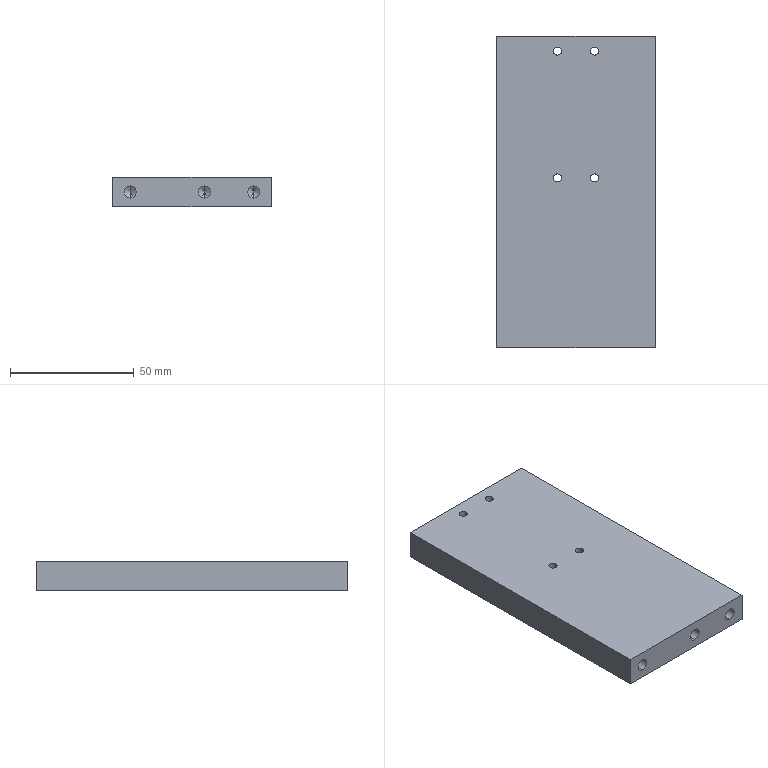Part | STEP file | PN_0018 tank-chain fixing block | 1 solid | 26 faces | box 64 x 126 x 12 mm | volume 95444 mm3 | cylinder 14 | cone 6 | plane 6 | commonest cylinder face diameters 3.3 x8 5 x6